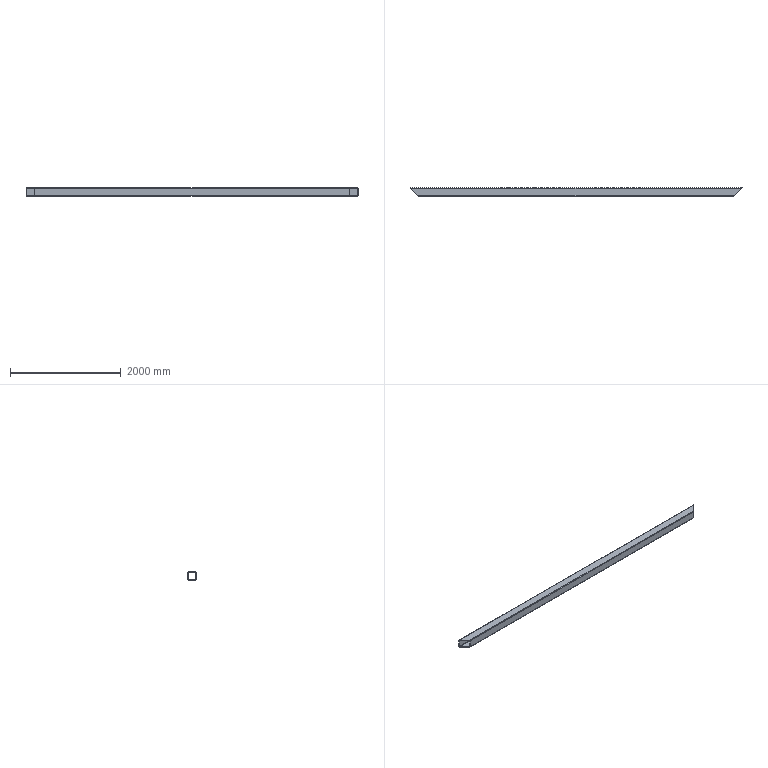Part | SolidWorks | features ICE 1, WeldMemberFeat 1, WeldmentFeature 1 | 1 solid | 18 faces | box 6000 x 150 x 150 mm | volume 16588374 mm3 | plane 10 | cylinder 8 | commonest cylinder face diameters 10 x4 20 x4
STEP:
#1=CARTESIAN_POINT('',(2990.,65.,75.));
#2=VERTEX_POINT('',#1);
#3=CARTESIAN_POINT('',(-2990.,65.,75.));
#4=VERTEX_POINT('',#3);
#5=CARTESIAN_POINT('',(3000.,65.,75.));
#6=DIRECTION('',(-1.,0.,0.));
#7=VECTOR('',#6,1000.);
#8=LINE('',#5,#7);
#9=EDGE_CURVE('',#2,#4,#8,.T.);
#10=ORIENTED_EDGE('',*,*,#9,.F.);
#11=CARTESIAN_POINT('',(3000.,75.,65.));
#12=VERTEX_POINT('',#11);
#13=CARTESIAN_POINT('',(2990.,65.,75.));
#14=CARTESIAN_POINT('',(2995.858,70.858,75.));
#15=CARTESIAN_POINT('',(3000.,75.,70.858));
#16=CARTESIAN_POINT('',(3000.,75.,65.));
#17=(BOUNDED_CURVE()B_SPLINE_CURVE(3,(#13,#14,#15,#16),.UNSPECIFIED.,.F.,.F.)B_SPLINE_CURVE_WITH_KNOTS((4,4),(1.571,3.142),.UNSPECIFIED.)CURVE()GEOMETRIC_REPRESENTATION_ITEM()RATIONAL_B_SPLINE_CURVE((1.,0.8047,0.8047,1.))REPRESENTATION_ITEM(''));
#18=EDGE_CURVE('',#2,#12,#17,.T.);
#19=ORIENTED_EDGE('',*,*,#18,.T.);
#20=CARTESIAN_POINT('',(-3000.,75.,65.));
#21=VERTEX_POINT('',#20);
#22=CARTESIAN_POINT('',(3000.,75.,65.));
#23=DIRECTION('',(-1.,0.,0.));
#24=VECTOR('',#23,1000.);
#25=LINE('',#22,#24);
#26=EDGE_CURVE('',#12,#21,#25,.T.);
#27=ORIENTED_EDGE('',*,*,#26,.T.);
#28=CARTESIAN_POINT('',(-3000.,75.,65.));
#29=CARTESIAN_POINT('',(-3000.,75.,70.858));
#30=CARTESIAN_POINT('',(-2995.858,70.858,75.));
#31=CARTESIAN_POINT('',(-2990.,65.,75.));
#32=(BOUNDED_CURVE()B_SPLINE_CURVE(3,(#28,#29,#30,#31),.UNSPECIFIED.,.F.,.F.)B_SPLINE_CURVE_WITH_KNOTS((4,4),(0.,1.571),.UNSPECIFIED.)CURVE()GEOMETRIC_REPRESENTATION_ITEM()RATIONAL_B_SPLINE_CURVE((1.,0.8047,0.8047,1.))REPRESENTATION_ITEM(''));
#33=EDGE_CURVE('',#21,#4,#32,.T.);
#34=ORIENTED_EDGE('',*,*,#33,.T.);
#35=EDGE_LOOP('',(#10,#19,#27,#34));
#36=FACE_OUTER_BOUND('',#35,.T.);
#37=CARTESIAN_POINT('',(3000.,65.,65.));
#38=DIRECTION('',(-1.,0.,0.));
#39=DIRECTION('',(0.,0.,1.));
#40=AXIS2_PLACEMENT_3D('',#37,#38,#39);
#41=CYLINDRICAL_SURFACE('',#40,10.);
#42=ADVANCED_FACE('',(#36),#41,.T.);
#43=CARTESIAN_POINT('',(2860.,-65.,75.));
#44=VERTEX_POINT('',#43);
#45=CARTESIAN_POINT('',(-2860.,-65.,75.));
#46=VERTEX_POINT('',#45);
#47=CARTESIAN_POINT('',(3000.,-65.,75.));
#48=DIRECTION('',(-1.,0.,0.));
#49=VECTOR('',#48,1000.);
#50=LINE('',#47,#49);
#51=EDGE_CURVE('',#44,#46,#50,.T.);
#52=ORIENTED_EDGE('',*,*,#51,.F.);
#53=CARTESIAN_POINT('',(2850.,-75.,75.));
#54=DIRECTION('',(0.7071,0.7071,0.));
#55=VECTOR('',#54,1000.);
#56=LINE('',#53,#55);
#57=EDGE_CURVE('',#44,#2,#56,.T.);
#58=ORIENTED_EDGE('',*,*,#57,.T.);
#59=ORIENTED_EDGE('',*,*,#9,.T.);
#60=CARTESIAN_POINT('',(-2850.,-75.,75.));
#61=DIRECTION('',(0.7071,-0.7071,0.));
#62=VECTOR('',#61,1000.);
#63=LINE('',#60,#62);
#64=EDGE_CURVE('',#4,#46,#63,.T.);
#65=ORIENTED_EDGE('',*,*,#64,.T.);
#66=EDGE_LOOP('',(#52,#58,#59,#65));
#67=FACE_OUTER_BOUND('',#66,.T.);
#68=CARTESIAN_POINT('',(3000.,65.,75.));
#69=DIRECTION('',(0.,0.,-1.));
#70=DIRECTION('',(-1.,0.,0.));
#71=AXIS2_PLACEMENT_3D('',#68,#69,#70);
#72=PLANE('',#71);
#73=ADVANCED_FACE('',(#67),#72,.F.);
#74=CARTESIAN_POINT('',(2850.,-75.,65.));
#75=VERTEX_POINT('',#74);
#76=CARTESIAN_POINT('',(-2850.,-75.,65.));
#77=VERTEX_POINT('',#76);
#78=CARTESIAN_POINT('',(3000.,-75.,65.));
#79=DIRECTION('',(-1.,0.,0.));
#80=VECTOR('',#79,1000.);
#81=LINE('',#78,#80);
#82=EDGE_CURVE('',#75,#77,#81,.T.);
#83=ORIENTED_EDGE('',*,*,#82,.F.);
#84=CARTESIAN_POINT('',(2850.,-75.,65.));
#85=CARTESIAN_POINT('',(2850.,-75.,70.858));
#86=CARTESIAN_POINT('',(2854.142,-70.858,75.));
#87=CARTESIAN_POINT('',(2860.,-65.,75.));
#88=(BOUNDED_CURVE()B_SPLINE_CURVE(3,(#84,#85,#86,#87),.UNSPECIFIED.,.F.,.F.)B_SPLINE_CURVE_WITH_KNOTS((4,4),(0.,1.571),.UNSPECIFIED.)CURVE()GEOMETRIC_REPRESENTATION_ITEM()RATIONAL_B_SPLINE_CURVE((1.,0.8047,0.8047,1.))REPRESENTATION_ITEM(''));
#89=EDGE_CURVE('',#75,#44,#88,.T.);
#90=ORIENTED_EDGE('',*,*,#89,.T.);
#91=ORIENTED_EDGE('',*,*,#51,.T.);
#92=CARTESIAN_POINT('',(-2860.,-65.,75.));
#93=CARTESIAN_POINT('',(-2854.142,-70.858,75.));
#94=CARTESIAN_POINT('',(-2850.,-75.,70.858));
#95=CARTESIAN_POINT('',(-2850.,-75.,65.));
#96=(BOUNDED_CURVE()B_SPLINE_CURVE(3,(#92,#93,#94,#95),.UNSPECIFIED.,.F.,.F.)B_SPLINE_CURVE_WITH_KNOTS((4,4),(1.571,3.142),.UNSPECIFIED.)CURVE()GEOMETRIC_REPRESENTATION_ITEM()RATIONAL_B_SPLINE_CURVE((1.,0.8047,0.8047,1.))REPRESENTATION_ITEM(''));
#97=EDGE_CURVE('',#46,#77,#96,.T.);
#98=ORIENTED_EDGE('',*,*,#97,.T.);
#99=EDGE_LOOP('',(#83,#90,#91,#98));
#100=FACE_OUTER_BOUND('',#99,.T.);
#101=CARTESIAN_POINT('',(3000.,-65.,65.));
#102=DIRECTION('',(-1.,0.,0.));
#103=DIRECTION('',(0.,0.,1.));
#104=AXIS2_PLACEMENT_3D('',#101,#102,#103);
#105=CYLINDRICAL_SURFACE('',#104,10.);
#106=ADVANCED_FACE('',(#100),#105,.T.);
#107=CARTESIAN_POINT('',(2850.,-75.,-65.));
#108=VERTEX_POINT('',#107);
#109=CARTESIAN_POINT('',(-2850.,-75.,-65.));
#110=VERTEX_POINT('',#109);
#111=CARTESIAN_POINT('',(3000.,-75.,-65.));
#112=DIRECTION('',(-1.,0.,0.));
#113=VECTOR('',#112,1000.);
#114=LINE('',#111,#113);
#115=EDGE_CURVE('',#108,#110,#114,.T.);
#116=ORIENTED_EDGE('',*,*,#115,.F.);
#117=CARTESIAN_POINT('',(2850.,-75.,75.));
#118=DIRECTION('',(0.,0.,-1.));
#119=VECTOR('',#118,1000.);
#120=LINE('',#117,#119);
#121=EDGE_CURVE('',#75,#108,#120,.T.);
#122=ORIENTED_EDGE('',*,*,#121,.F.);
#123=ORIENTED_EDGE('',*,*,#82,.T.);
#124=CARTESIAN_POINT('',(-2850.,-75.,75.));
#125=DIRECTION('',(0.,0.,-1.));
#126=VECTOR('',#125,1000.);
#127=LINE('',#124,#126);
#128=EDGE_CURVE('',#77,#110,#127,.T.);
#129=ORIENTED_EDGE('',*,*,#128,.T.);
#130=EDGE_LOOP('',(#116,#122,#123,#129));
#131=FACE_OUTER_BOUND('',#130,.T.);
#132=CARTESIAN_POINT('',(3000.,-75.,-65.));
#133=DIRECTION('',(0.,1.,0.));
#134=DIRECTION('',(0.,0.,1.));
#135=AXIS2_PLACEMENT_3D('',#132,#133,#134);
#136=PLANE('',#135);
#137=ADVANCED_FACE('',(#131),#136,.F.);
#138=CARTESIAN_POINT('',(2860.,-65.,-75.));
#139=VERTEX_POINT('',#138);
#140=CARTESIAN_POINT('',(-2860.,-65.,-75.));
#141=VERTEX_POINT('',#140);
#142=CARTESIAN_POINT('',(3000.,-65.,-75.));
#143=DIRECTION('',(-1.,0.,0.));
#144=VECTOR('',#143,1000.);
#145=LINE('',#142,#144);
#146=EDGE_CURVE('',#139,#141,#145,.T.);
#147=ORIENTED_EDGE('',*,*,#146,.F.);
#148=CARTESIAN_POINT('',(2860.,-65.,-75.));
#149=CARTESIAN_POINT('',(2854.142,-70.858,-75.));
#150=CARTESIAN_POINT('',(2850.,-75.,-70.858));
#151=CARTESIAN_POINT('',(2850.,-75.,-65.));
#152=(BOUNDED_CURVE()B_SPLINE_CURVE(3,(#148,#149,#150,#151),.UNSPECIFIED.,.F.,.T.)B_SPLINE_CURVE_WITH_KNOTS((4,4),(4.712,6.283),.UNSPECIFIED.)CURVE()GEOMETRIC_REPRESENTATION_ITEM()RATIONAL_B_SPLINE_CURVE((1.,0.8047,0.8047,1.))REPRESENTATION_ITEM(''));
#153=EDGE_CURVE('',#139,#108,#152,.T.);
#154=ORIENTED_EDGE('',*,*,#153,.T.);
#155=ORIENTED_EDGE('',*,*,#115,.T.);
#156=CARTESIAN_POINT('',(-2850.,-75.,-65.));
#157=CARTESIAN_POINT('',(-2850.,-75.,-70.858));
#158=CARTESIAN_POINT('',(-2854.142,-70.858,-75.));
#159=CARTESIAN_POINT('',(-2860.,-65.,-75.));
#160=(BOUNDED_CURVE()B_SPLINE_CURVE(3,(#156,#157,#158,#159),.UNSPECIFIED.,.F.,.F.)B_SPLINE_CURVE_WITH_KNOTS((4,4),(3.142,4.712),.UNSPECIFIED.)CURVE()GEOMETRIC_REPRESENTATION_ITEM()RATIONAL_B_SPLINE_CURVE((1.,0.8047,0.8047,1.))REPRESENTATION_ITEM(''));
#161=EDGE_CURVE('',#110,#141,#160,.T.);
#162=ORIENTED_EDGE('',*,*,#161,.T.);
#163=EDGE_LOOP('',(#147,#154,#155,#162));
#164=FACE_OUTER_BOUND('',#163,.T.);
#165=CARTESIAN_POINT('',(3000.,-65.,-65.));
#166=DIRECTION('',(-1.,0.,0.));
#167=DIRECTION('',(0.,0.,1.));
#168=AXIS2_PLACEMENT_3D('',#165,#166,#167);
#169=CYLINDRICAL_SURFACE('',#168,10.);
#170=ADVANCED_FACE('',(#164),#169,.T.);
#171=CARTESIAN_POINT('',(2990.,65.,-75.));
#172=VERTEX_POINT('',#171);
#173=CARTESIAN_POINT('',(-2990.,65.,-75.));
#174=VERTEX_POINT('',#173);
#175=CARTESIAN_POINT('',(3000.,65.,-75.));
#176=DIRECTION('',(-1.,0.,0.));
#177=VECTOR('',#176,1000.);
#178=LINE('',#175,#177);
#179=EDGE_CURVE('',#172,#174,#178,.T.);
#180=ORIENTED_EDGE('',*,*,#179,.F.);
#181=CARTESIAN_POINT('',(2850.,-75.,-75.));
#182=DIRECTION('',(0.7071,0.7071,0.));
#183=VECTOR('',#182,1000.);
#184=LINE('',#181,#183);
#185=EDGE_CURVE('',#139,#172,#184,.T.);
#186=ORIENTED_EDGE('',*,*,#185,.F.);
#187=ORIENTED_EDGE('',*,*,#146,.T.);
#188=CARTESIAN_POINT('',(-2850.,-75.,-75.));
#189=DIRECTION('',(0.7071,-0.7071,0.));
#190=VECTOR('',#189,1000.);
#191=LINE('',#188,#190);
#192=EDGE_CURVE('',#174,#141,#191,.T.);
#193=ORIENTED_EDGE('',*,*,#192,.F.);
#194=EDGE_LOOP('',(#180,#186,#187,#193));
#195=FACE_OUTER_BOUND('',#194,.T.);
#196=CARTESIAN_POINT('',(3000.,-65.,-75.));
#197=DIRECTION('',(0.,0.,1.));
#198=DIRECTION('',(1.,0.,0.));
#199=AXIS2_PLACEMENT_3D('',#196,#197,#198);
#200=PLANE('',#199);
#201=ADVANCED_FACE('',(#195),#200,.F.);
#202=CARTESIAN_POINT('',(3000.,75.,-65.));
#203=VERTEX_POINT('',#202);
#204=CARTESIAN_POINT('',(-3000.,75.,-65.));
#205=VERTEX_POINT('',#204);
#206=CARTESIAN_POINT('',(3000.,75.,-65.));
#207=DIRECTION('',(-1.,0.,0.));
#208=VECTOR('',#207,1000.);
#209=LINE('',#206,#208);
#210=EDGE_CURVE('',#203,#205,#209,.T.);
#211=ORIENTED_EDGE('',*,*,#210,.F.);
#212=CARTESIAN_POINT('',(3000.,75.,-65.));
#213=CARTESIAN_POINT('',(3000.,75.,-70.858));
#214=CARTESIAN_POINT('',(2995.858,70.858,-75.));
#215=CARTESIAN_POINT('',(2990.,65.,-75.));
#216=(BOUNDED_CURVE()B_SPLINE_CURVE(3,(#212,#213,#214,#215),.UNSPECIFIED.,.F.,.F.)B_SPLINE_CURVE_WITH_KNOTS((4,4),(3.142,4.712),.UNSPECIFIED.)CURVE()GEOMETRIC_REPRESENTATION_ITEM()RATIONAL_B_SPLINE_CURVE((1.,0.8047,0.8047,1.))REPRESENTATION_ITEM(''));
#217=EDGE_CURVE('',#203,#172,#216,.T.);
#218=ORIENTED_EDGE('',*,*,#217,.T.);
#219=ORIENTED_EDGE('',*,*,#179,.T.);
#220=CARTESIAN_POINT('',(-2990.,65.,-75.));
#221=CARTESIAN_POINT('',(-2995.858,70.858,-75.));
#222=CARTESIAN_POINT('',(-3000.,75.,-70.858));
#223=CARTESIAN_POINT('',(-3000.,75.,-65.));
#224=(BOUNDED_CURVE()B_SPLINE_CURVE(3,(#220,#221,#222,#223),.UNSPECIFIED.,.F.,.F.)B_SPLINE_CURVE_WITH_KNOTS((4,4),(4.712,6.283),.UNSPECIFIED.)CURVE()GEOMETRIC_REPRESENTATION_ITEM()RATIONAL_B_SPLINE_CURVE((1.,0.8047,0.8047,1.))REPRESENTATION_ITEM(''));
#225=EDGE_CURVE('',#174,#205,#224,.T.);
#226=ORIENTED_EDGE('',*,*,#225,.T.);
#227=EDGE_LOOP('',(#211,#218,#219,#226));
#228=FACE_OUTER_BOUND('',#227,.T.);
#229=CARTESIAN_POINT('',(3000.,65.,-65.));
#230=DIRECTION('',(-1.,0.,0.));
#231=DIRECTION('',(0.,0.,1.));
#232=AXIS2_PLACEMENT_3D('',#229,#230,#231);
#233=CYLINDRICAL_SURFACE('',#232,10.);
#234=ADVANCED_FACE('',(#228),#233,.T.);
#235=CARTESIAN_POINT('',(2855.,-70.,65.));
#236=VERTEX_POINT('',#235);
#237=CARTESIAN_POINT('',(2860.,-65.,70.));
#238=VERTEX_POINT('',#237);
#239=CARTESIAN_POINT('',(2855.,-70.,65.));
#240=CARTESIAN_POINT('',(2855.,-70.,67.929));
#241=CARTESIAN_POINT('',(2857.071,-67.929,70.));
#242=CARTESIAN_POINT('',(2860.,-65.,70.));
#243=(BOUNDED_CURVE()B_SPLINE_CURVE(3,(#239,#240,#241,#242),.UNSPECIFIED.,.F.,.F.)B_SPLINE_CURVE_WITH_KNOTS((4,4),(0.,1.571),.UNSPECIFIED.)CURVE()GEOMETRIC_REPRESENTATION_ITEM()RATIONAL_B_SPLINE_CURVE((1.,0.8047,0.8047,1.))REPRESENTATION_ITEM(''));
#244=EDGE_CURVE('',#236,#238,#243,.T.);
#245=ORIENTED_EDGE('',*,*,#244,.F.);
#246=CARTESIAN_POINT('',(-2855.,-70.,65.));
#247=VERTEX_POINT('',#246);
#248=CARTESIAN_POINT('',(3000.,-70.,65.));
#249=DIRECTION('',(-1.,0.,0.));
#250=VECTOR('',#249,1000.);
#251=LINE('',#248,#250);
#252=EDGE_CURVE('',#236,#247,#251,.T.);
#253=ORIENTED_EDGE('',*,*,#252,.T.);
#254=CARTESIAN_POINT('',(-2860.,-65.,70.));
#255=VERTEX_POINT('',#254);
#256=CARTESIAN_POINT('',(-2860.,-65.,70.));
#257=CARTESIAN_POINT('',(-2857.071,-67.929,70.));
#258=CARTESIAN_POINT('',(-2855.,-70.,67.929));
#259=CARTESIAN_POINT('',(-2855.,-70.,65.));
#260=(BOUNDED_CURVE()B_SPLINE_CURVE(3,(#256,#257,#258,#259),.UNSPECIFIED.,.F.,.F.)B_SPLINE_CURVE_WITH_KNOTS((4,4),(1.571,3.142),.UNSPECIFIED.)CURVE()GEOMETRIC_REPRESENTATION_ITEM()RATIONAL_B_SPLINE_CURVE((1.,0.8047,0.8047,1.))REPRESENTATION_ITEM(''));
#261=EDGE_CURVE('',#255,#247,#260,.T.);
#262=ORIENTED_EDGE('',*,*,#261,.F.);
#263=CARTESIAN_POINT('',(3000.,-65.,70.));
#264=DIRECTION('',(-1.,0.,0.));
#265=VECTOR('',#264,1000.);
#266=LINE('',#263,#265);
#267=EDGE_CURVE('',#238,#255,#266,.T.);
#268=ORIENTED_EDGE('',*,*,#267,.F.);
#269=EDGE_LOOP('',(#245,#253,#262,#268));
#270=FACE_OUTER_BOUND('',#269,.T.);
#271=CARTESIAN_POINT('',(3000.,-65.,65.));
#272=DIRECTION('',(-1.,0.,0.));
#273=DIRECTION('',(0.,0.,1.));
#274=AXIS2_PLACEMENT_3D('',#271,#272,#273);
#275=CYLINDRICAL_SURFACE('',#274,5.);
#276=ADVANCED_FACE('',(#270),#275,.F.);
#277=CARTESIAN_POINT('',(2990.,65.,70.));
#278=VERTEX_POINT('',#277);
#279=CARTESIAN_POINT('',(2995.,70.,70.));
#280=DIRECTION('',(0.7071,0.7071,0.));
#281=VECTOR('',#280,1000.);
#282=LINE('',#279,#281);
#283=EDGE_CURVE('',#238,#278,#282,.T.);
#284=ORIENTED_EDGE('',*,*,#283,.F.);
#285=ORIENTED_EDGE('',*,*,#267,.T.);
#286=CARTESIAN_POINT('',(-2990.,65.,70.));
#287=VERTEX_POINT('',#286);
#288=CARTESIAN_POINT('',(5.,-2930.,70.));
#289=DIRECTION('',(0.7071,-0.7071,0.));
#290=VECTOR('',#289,1000.);
#291=LINE('',#288,#290);
#292=EDGE_CURVE('',#287,#255,#291,.T.);
#293=ORIENTED_EDGE('',*,*,#292,.F.);
#294=CARTESIAN_POINT('',(3000.,65.,70.));
#295=DIRECTION('',(-1.,0.,0.));
#296=VECTOR('',#295,1000.);
#297=LINE('',#294,#296);
#298=EDGE_CURVE('',#278,#287,#297,.T.);
#299=ORIENTED_EDGE('',*,*,#298,.F.);
#300=EDGE_LOOP('',(#284,#285,#293,#299));
#301=FACE_OUTER_BOUND('',#300,.T.);
#302=CARTESIAN_POINT('',(3000.,65.,70.));
#303=DIRECTION('',(0.,0.,-1.));
#304=DIRECTION('',(-1.,0.,0.));
#305=AXIS2_PLACEMENT_3D('',#302,#303,#304);
#306=PLANE('',#305);
#307=ADVANCED_FACE('',(#301),#306,.T.);
#308=CARTESIAN_POINT('',(2995.,70.,65.));
#309=VERTEX_POINT('',#308);
#310=CARTESIAN_POINT('',(2990.,65.,70.));
#311=CARTESIAN_POINT('',(2992.929,67.929,70.));
#312=CARTESIAN_POINT('',(2995.,70.,67.929));
#313=CARTESIAN_POINT('',(2995.,70.,65.));
#314=(BOUNDED_CURVE()B_SPLINE_CURVE(3,(#310,#311,#312,#313),.UNSPECIFIED.,.F.,.F.)B_SPLINE_CURVE_WITH_KNOTS((4,4),(1.571,3.142),.UNSPECIFIED.)CURVE()GEOMETRIC_REPRESENTATION_ITEM()RATIONAL_B_SPLINE_CURVE((1.,0.8047,0.8047,1.))REPRESENTATION_ITEM(''));
#315=EDGE_CURVE('',#278,#309,#314,.T.);
#316=ORIENTED_EDGE('',*,*,#315,.F.);
#317=ORIENTED_EDGE('',*,*,#298,.T.);
#318=CARTESIAN_POINT('',(-2995.,70.,65.));
#319=VERTEX_POINT('',#318);
#320=CARTESIAN_POINT('',(-2995.,70.,65.));
#321=CARTESIAN_POINT('',(-2995.,70.,67.929));
#322=CARTESIAN_POINT('',(-2992.929,67.929,70.));
#323=CARTESIAN_POINT('',(-2990.,65.,70.));
#324=(BOUNDED_CURVE()B_SPLINE_CURVE(3,(#320,#321,#322,#323),.UNSPECIFIED.,.F.,.F.)B_SPLINE_CURVE_WITH_KNOTS((4,4),(0.,1.571),.UNSPECIFIED.)CURVE()GEOMETRIC_REPRESENTATION_ITEM()RATIONAL_B_SPLINE_CURVE((1.,0.8047,0.8047,1.))REPRESENTATION_ITEM(''));
#325=EDGE_CURVE('',#319,#287,#324,.T.);
#326=ORIENTED_EDGE('',*,*,#325,.F.);
#327=CARTESIAN_POINT('',(3000.,70.,65.));
#328=DIRECTION('',(-1.,0.,0.));
#329=VECTOR('',#328,1000.);
#330=LINE('',#327,#329);
#331=EDGE_CURVE('',#309,#319,#330,.T.);
#332=ORIENTED_EDGE('',*,*,#331,.F.);
#333=EDGE_LOOP('',(#316,#317,#326,#332));
#334=FACE_OUTER_BOUND('',#333,.T.);
#335=CARTESIAN_POINT('',(3000.,65.,65.));
#336=DIRECTION('',(-1.,0.,0.));
#337=DIRECTION('',(0.,0.,1.));
#338=AXIS2_PLACEMENT_3D('',#335,#336,#337);
#339=CYLINDRICAL_SURFACE('',#338,5.);
#340=ADVANCED_FACE('',(#334),#339,.F.);
#341=CARTESIAN_POINT('',(2995.,70.,-65.));
#342=VERTEX_POINT('',#341);
#343=CARTESIAN_POINT('',(2995.,70.,65.));
#344=DIRECTION('',(0.,0.,-1.));
#345=VECTOR('',#344,1000.);
#346=LINE('',#343,#345);
#347=EDGE_CURVE('',#309,#342,#346,.T.);
#348=ORIENTED_EDGE('',*,*,#347,.F.);
#349=ORIENTED_EDGE('',*,*,#331,.T.);
#350=CARTESIAN_POINT('',(-2995.,70.,-65.));
#351=VERTEX_POINT('',#350);
#352=CARTESIAN_POINT('',(-2995.,70.,65.));
#353=DIRECTION('',(0.,0.,1.));
#354=VECTOR('',#353,1000.);
#355=LINE('',#352,#354);
#356=EDGE_CURVE('',#351,#319,#355,.T.);
#357=ORIENTED_EDGE('',*,*,#356,.F.);
#358=CARTESIAN_POINT('',(3000.,70.,-65.));
#359=DIRECTION('',(-1.,0.,0.));
#360=VECTOR('',#359,1000.);
#361=LINE('',#358,#360);
#362=EDGE_CURVE('',#342,#351,#361,.T.);
#363=ORIENTED_EDGE('',*,*,#362,.F.);
#364=EDGE_LOOP('',(#348,#349,#357,#363));
#365=FACE_OUTER_BOUND('',#364,.T.);
#366=CARTESIAN_POINT('',(3000.,70.,65.));
#367=DIRECTION('',(0.,-1.,0.));
#368=DIRECTION('',(0.,0.,-1.));
#369=AXIS2_PLACEMENT_3D('',#366,#367,#368);
#370=PLANE('',#369);
#371=ADVANCED_FACE('',(#365),#370,.T.);
#372=CARTESIAN_POINT('',(2990.,65.,-70.));
#373=VERTEX_POINT('',#372);
#374=CARTESIAN_POINT('',(2995.,70.,-65.));
#375=CARTESIAN_POINT('',(2995.,70.,-67.929));
#376=CARTESIAN_POINT('',(2992.929,67.929,-70.));
#377=CARTESIAN_POINT('',(2990.,65.,-70.));
#378=(BOUNDED_CURVE()B_SPLINE_CURVE(3,(#374,#375,#376,#377),.UNSPECIFIED.,.F.,.T.)B_SPLINE_CURVE_WITH_KNOTS((4,4),(3.142,4.712),.UNSPECIFIED.)CURVE()GEOMETRIC_REPRESENTATION_ITEM()RATIONAL_B_SPLINE_CURVE((1.,0.8047,0.8047,1.))REPRESENTATION_ITEM(''));
#379=EDGE_CURVE('',#342,#373,#378,.T.);
#380=ORIENTED_EDGE('',*,*,#379,.F.);
#381=ORIENTED_EDGE('',*,*,#362,.T.);
#382=CARTESIAN_POINT('',(-2990.,65.,-70.));
#383=VERTEX_POINT('',#382);
#384=CARTESIAN_POINT('',(-2990.,65.,-70.));
#385=CARTESIAN_POINT('',(-2992.929,67.929,-70.));
#386=CARTESIAN_POINT('',(-2995.,70.,-67.929));
#387=CARTESIAN_POINT('',(-2995.,70.,-65.));
#388=(BOUNDED_CURVE()B_SPLINE_CURVE(3,(#384,#385,#386,#387),.UNSPECIFIED.,.F.,.T.)B_SPLINE_CURVE_WITH_KNOTS((4,4),(4.712,6.283),.UNSPECIFIED.)CURVE()GEOMETRIC_REPRESENTATION_ITEM()RATIONAL_B_SPLINE_CURVE((1.,0.8047,0.8047,1.))REPRESENTATION_ITEM(''));
#389=EDGE_CURVE('',#383,#351,#388,.T.);
#390=ORIENTED_EDGE('',*,*,#389,.F.);
#391=CARTESIAN_POINT('',(3000.,65.,-70.));
#392=DIRECTION('',(-1.,0.,0.));
#393=VECTOR('',#392,1000.);
#394=LINE('',#391,#393);
#395=EDGE_CURVE('',#373,#383,#394,.T.);
#396=ORIENTED_EDGE('',*,*,#395,.F.);
#397=EDGE_LOOP('',(#380,#381,#390,#396));
#398=FACE_OUTER_BOUND('',#397,.T.);
#399=CARTESIAN_POINT('',(3000.,65.,-65.));
#400=DIRECTION('',(-1.,0.,0.));
#401=DIRECTION('',(0.,0.,1.));
#402=AXIS2_PLACEMENT_3D('',#399,#400,#401);
#403=CYLINDRICAL_SURFACE('',#402,5.);
#404=ADVANCED_FACE('',(#398),#403,.F.);
#405=CARTESIAN_POINT('',(2860.,-65.,-70.));
#406=VERTEX_POINT('',#405);
#407=CARTESIAN_POINT('',(2930.,5.,-70.));
#408=DIRECTION('',(-0.7071,-0.7071,0.));
#409=VECTOR('',#408,1000.);
#410=LINE('',#407,#409);
#411=EDGE_CURVE('',#373,#406,#410,.T.);
#412=ORIENTED_EDGE('',*,*,#411,.F.);
#413=ORIENTED_EDGE('',*,*,#395,.T.);
#414=CARTESIAN_POINT('',(-2860.,-65.,-70.));
#415=VERTEX_POINT('',#414);
#416=CARTESIAN_POINT('',(70.,-2995.,-70.));
#417=DIRECTION('',(-0.7071,0.7071,0.));
#418=VECTOR('',#417,1000.);
#419=LINE('',#416,#418);
#420=EDGE_CURVE('',#415,#383,#419,.T.);
#421=ORIENTED_EDGE('',*,*,#420,.F.);
#422=CARTESIAN_POINT('',(3000.,-65.,-70.));
#423=DIRECTION('',(-1.,0.,0.));
#424=VECTOR('',#423,1000.);
#425=LINE('',#422,#424);
#426=EDGE_CURVE('',#406,#415,#425,.T.);
#427=ORIENTED_EDGE('',*,*,#426,.F.);
#428=EDGE_LOOP('',(#412,#413,#421,#427));
#429=FACE_OUTER_BOUND('',#428,.T.);
#430=CARTESIAN_POINT('',(3000.,-65.,-70.));
#431=DIRECTION('',(0.,0.,1.));
#432=DIRECTION('',(1.,0.,0.));
#433=AXIS2_PLACEMENT_3D('',#430,#431,#432);
#434=PLANE('',#433);
#435=ADVANCED_FACE('',(#429),#434,.T.);
#436=CARTESIAN_POINT('',(2855.,-70.,-65.));
#437=VERTEX_POINT('',#436);
#438=CARTESIAN_POINT('',(2860.,-65.,-70.));
#439=CARTESIAN_POINT('',(2857.071,-67.929,-70.));
#440=CARTESIAN_POINT('',(2855.,-70.,-67.929));
#441=CARTESIAN_POINT('',(2855.,-70.,-65.));
#442=(BOUNDED_CURVE()B_SPLINE_CURVE(3,(#438,#439,#440,#441),.UNSPECIFIED.,.F.,.F.)B_SPLINE_CURVE_WITH_KNOTS((4,4),(4.712,6.283),.UNSPECIFIED.)CURVE()GEOMETRIC_REPRESENTATION_ITEM()RATIONAL_B_SPLINE_CURVE((1.,0.8047,0.8047,1.))REPRESENTATION_ITEM(''));
#443=EDGE_CURVE('',#406,#437,#442,.T.);
#444=ORIENTED_EDGE('',*,*,#443,.F.);
#445=ORIENTED_EDGE('',*,*,#426,.T.);
#446=CARTESIAN_POINT('',(-2855.,-70.,-65.));
#447=VERTEX_POINT('',#446);
#448=CARTESIAN_POINT('',(-2855.,-70.,-65.));
#449=CARTESIAN_POINT('',(-2855.,-70.,-67.929));
#450=CARTESIAN_POINT('',(-2857.071,-67.929,-70.));
#451=CARTESIAN_POINT('',(-2860.,-65.,-70.));
#452=(BOUNDED_CURVE()B_SPLINE_CURVE(3,(#448,#449,#450,#451),.UNSPECIFIED.,.F.,.F.)B_SPLINE_CURVE_WITH_KNOTS((4,4),(3.142,4.712),.UNSPECIFIED.)CURVE()GEOMETRIC_REPRESENTATION_ITEM()RATIONAL_B_SPLINE_CURVE((1.,0.8047,0.8047,1.))REPRESENTATION_ITEM(''));
#453=EDGE_CURVE('',#447,#415,#452,.T.);
#454=ORIENTED_EDGE('',*,*,#453,.F.);
#455=CARTESIAN_POINT('',(3000.,-70.,-65.));
#456=DIRECTION('',(-1.,0.,0.));
#457=VECTOR('',#456,1000.);
#458=LINE('',#455,#457);
#459=EDGE_CURVE('',#437,#447,#458,.T.);
#460=ORIENTED_EDGE('',*,*,#459,.F.);
#461=EDGE_LOOP('',(#444,#445,#454,#460));
#462=FACE_OUTER_BOUND('',#461,.T.);
#463=CARTESIAN_POINT('',(3000.,-65.,-65.));
#464=DIRECTION('',(-1.,0.,0.));
#465=DIRECTION('',(0.,0.,1.));
#466=AXIS2_PLACEMENT_3D('',#463,#464,#465);
#467=CYLINDRICAL_SURFACE('',#466,5.);
#468=ADVANCED_FACE('',(#462),#467,.F.);
#469=CARTESIAN_POINT('',(2855.,-70.,-65.));
#470=DIRECTION('',(0.,0.,1.));
#471=VECTOR('',#470,1000.);
#472=LINE('',#469,#471);
#473=EDGE_CURVE('',#437,#236,#472,.T.);
#474=ORIENTED_EDGE('',*,*,#473,.F.);
#475=ORIENTED_EDGE('',*,*,#459,.T.);
#476=CARTESIAN_POINT('',(-2855.,-70.,-65.));
#477=DIRECTION('',(0.,0.,-1.));
#478=VECTOR('',#477,1000.);
#479=LINE('',#476,#478);
#480=EDGE_CURVE('',#247,#447,#479,.T.);
#481=ORIENTED_EDGE('',*,*,#480,.F.);
#482=ORIENTED_EDGE('',*,*,#252,.F.);
#483=EDGE_LOOP('',(#474,#475,#481,#482));
#484=FACE_OUTER_BOUND('',#483,.T.);
#485=CARTESIAN_POINT('',(3000.,-70.,-65.));
#486=DIRECTION('',(0.,1.,0.));
#487=DIRECTION('',(0.,0.,1.));
#488=AXIS2_PLACEMENT_3D('',#485,#486,#487);
#489=PLANE('',#488);
#490=ADVANCED_FACE('',(#484),#489,.T.);
#491=CARTESIAN_POINT('',(-3000.,75.,65.));
#492=DIRECTION('',(0.,0.,1.));
#493=VECTOR('',#492,1000.);
#494=LINE('',#491,#493);
#495=EDGE_CURVE('',#205,#21,#494,.T.);
#496=ORIENTED_EDGE('',*,*,#495,.T.);
#497=ORIENTED_EDGE('',*,*,#26,.F.);
#498=CARTESIAN_POINT('',(3000.,75.,65.));
#499=DIRECTION('',(0.,0.,1.));
#500=VECTOR('',#499,1000.);
#501=LINE('',#498,#500);
#502=EDGE_CURVE('',#203,#12,#501,.T.);
#503=ORIENTED_EDGE('',*,*,#502,.F.);
#504=ORIENTED_EDGE('',*,*,#210,.T.);
#505=EDGE_LOOP('',(#496,#497,#503,#504));
#506=FACE_OUTER_BOUND('',#505,.T.);
#507=CARTESIAN_POINT('',(3000.,75.,65.));
#508=DIRECTION('',(0.,-1.,0.));
#509=DIRECTION('',(0.,0.,-1.));
#510=AXIS2_PLACEMENT_3D('',#507,#508,#509);
#511=PLANE('',#510);
#512=ADVANCED_FACE('',(#506),#511,.F.);
#513=ORIENTED_EDGE('',*,*,#261,.T.);
#514=ORIENTED_EDGE('',*,*,#480,.T.);
#515=ORIENTED_EDGE('',*,*,#453,.T.);
#516=ORIENTED_EDGE('',*,*,#420,.T.);
#517=ORIENTED_EDGE('',*,*,#389,.T.);
#518=ORIENTED_EDGE('',*,*,#356,.T.);
#519=ORIENTED_EDGE('',*,*,#325,.T.);
#520=ORIENTED_EDGE('',*,*,#292,.T.);
#521=EDGE_LOOP('',(#513,#514,#515,#516,#517,#518,#519,#520));
#522=FACE_BOUND('',#521,.T.);
#523=ORIENTED_EDGE('',*,*,#495,.F.);
#524=ORIENTED_EDGE('',*,*,#225,.F.);
#525=ORIENTED_EDGE('',*,*,#192,.T.);
#526=ORIENTED_EDGE('',*,*,#161,.F.);
#527=ORIENTED_EDGE('',*,*,#128,.F.);
#528=ORIENTED_EDGE('',*,*,#97,.F.);
#529=ORIENTED_EDGE('',*,*,#64,.F.);
#530=ORIENTED_EDGE('',*,*,#33,.F.);
#531=EDGE_LOOP('',(#523,#524,#525,#526,#527,#528,#529,#530));
#532=FACE_OUTER_BOUND('',#531,.T.);
#533=CARTESIAN_POINT('',(-2850.,-75.,75.));
#534=DIRECTION('',(0.7071,0.7071,0.));
#535=DIRECTION('',(-0.7071,0.7071,0.));
#536=AXIS2_PLACEMENT_3D('',#533,#534,#535);
#537=PLANE('',#536);
#538=ADVANCED_FACE('',(#522,#532),#537,.F.);
#539=ORIENTED_EDGE('',*,*,#244,.T.);
#540=ORIENTED_EDGE('',*,*,#283,.T.);
#541=ORIENTED_EDGE('',*,*,#315,.T.);
#542=ORIENTED_EDGE('',*,*,#347,.T.);
#543=ORIENTED_EDGE('',*,*,#379,.T.);
#544=ORIENTED_EDGE('',*,*,#411,.T.);
#545=ORIENTED_EDGE('',*,*,#443,.T.);
#546=ORIENTED_EDGE('',*,*,#473,.T.);
#547=EDGE_LOOP('',(#539,#540,#541,#542,#543,#544,#545,#546));
#548=FACE_BOUND('',#547,.T.);
#549=ORIENTED_EDGE('',*,*,#57,.F.);
#550=ORIENTED_EDGE('',*,*,#89,.F.);
#551=ORIENTED_EDGE('',*,*,#121,.T.);
#552=ORIENTED_EDGE('',*,*,#153,.F.);
#553=ORIENTED_EDGE('',*,*,#185,.T.);
#554=ORIENTED_EDGE('',*,*,#217,.F.);
#555=ORIENTED_EDGE('',*,*,#502,.T.);
#556=ORIENTED_EDGE('',*,*,#18,.F.);
#557=EDGE_LOOP('',(#549,#550,#551,#552,#553,#554,#555,#556));
#558=FACE_OUTER_BOUND('',#557,.T.);
#559=CARTESIAN_POINT('',(2850.,-75.,75.));
#560=DIRECTION('',(-0.7071,0.7071,0.));
#561=DIRECTION('',(-0.7071,-0.7071,0.));
#562=AXIS2_PLACEMENT_3D('',#559,#560,#561);
#563=PLANE('',#562);
#564=ADVANCED_FACE('',(#548,#558),#563,.F.);
#565=CLOSED_SHELL('',(#42,#73,#106,#137,#170,#201,#234,#276,#307,#340,#371,#404,#435,#468,#490,#512,#538,#564));
#566=MANIFOLD_SOLID_BREP('',#565);
#567=CARTESIAN_POINT('',(0.,0.,0.));
#568=DIRECTION('',(0.,0.,1.));
#569=DIRECTION('',(1.,0.,0.));
#570=AXIS2_PLACEMENT_3D('',#567,#568,#569);
#571=(LENGTH_UNIT()NAMED_UNIT(*)SI_UNIT(.MILLI.,.METRE.));
#572=UNCERTAINTY_MEASURE_WITH_UNIT(LENGTH_MEASURE(0.00001),#571,'','');
#573=(NAMED_UNIT(*)PLANE_ANGLE_UNIT()SI_UNIT($,.RADIAN.));
#574=(NAMED_UNIT(*)SI_UNIT($,.STERADIAN.)SOLID_ANGLE_UNIT());
#575=(GEOMETRIC_REPRESENTATION_CONTEXT(3)GLOBAL_UNCERTAINTY_ASSIGNED_CONTEXT((#572))GLOBAL_UNIT_ASSIGNED_CONTEXT((#571,#573,#574))REPRESENTATION_CONTEXT('',''));
#576=ADVANCED_BREP_SHAPE_REPRESENTATION('',(#566,#570),#575);